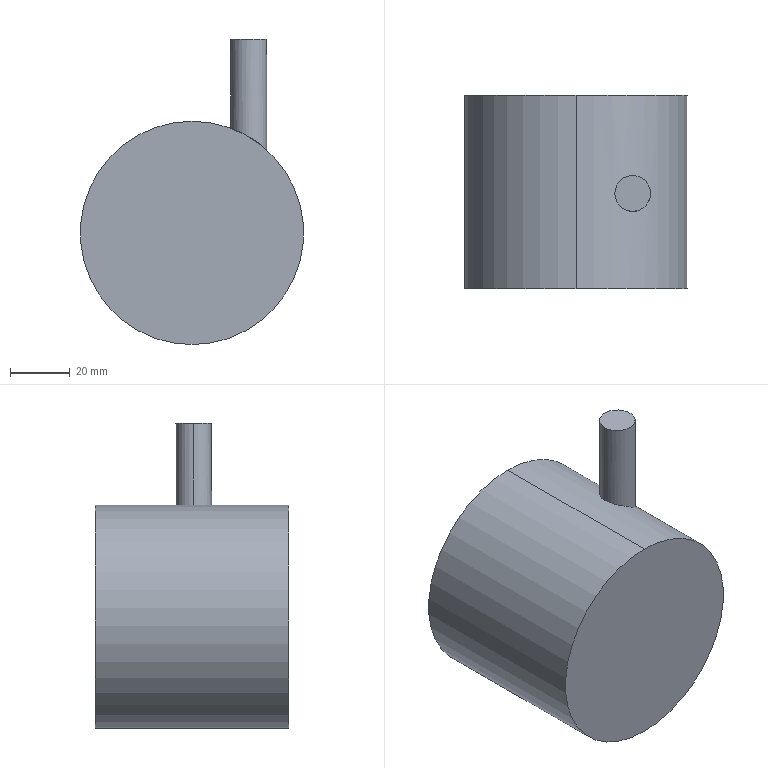Part | SolidWorks | features Extrusion 1, ICE 1 | 1 solid | 7 faces | box 75 x 65 x 102.5 mm | volume 290882 mm3 | cylinder 4 | plane 3 | commonest cylinder face diameters 12 x2 75 x2
STEP:
#1=CARTESIAN_POINT('',(25.06,31.933,65.));
#2=VERTEX_POINT('',#1);
#3=CARTESIAN_POINT('',(13.06,31.933,65.));
#4=VERTEX_POINT('',#3);
#5=CARTESIAN_POINT('',(19.06,31.933,65.));
#6=DIRECTION('',(0.,0.,1.));
#7=DIRECTION('',(1.,0.,0.));
#8=AXIS2_PLACEMENT_3D('',#5,#6,#7);
#9=CIRCLE('',#8,6.);
#10=EDGE_CURVE('',#2,#4,#9,.T.);
#11=ORIENTED_EDGE('',*,*,#10,.F.);
#12=CARTESIAN_POINT('',(25.06,31.933,27.897));
#13=VERTEX_POINT('',#12);
#14=CARTESIAN_POINT('',(25.06,31.933,65.));
#15=DIRECTION('',(0.,0.,-1.));
#16=VECTOR('',#15,1000.);
#17=LINE('',#14,#16);
#18=EDGE_CURVE('',#2,#13,#17,.T.);
#19=ORIENTED_EDGE('',*,*,#18,.T.);
#20=CARTESIAN_POINT('',(13.06,31.933,35.152));
#21=VERTEX_POINT('',#20);
#22=CARTESIAN_POINT('',(25.06,31.933,27.897));
#23=CARTESIAN_POINT('',(25.06,32.147,27.897));
#24=CARTESIAN_POINT('',(25.048,32.362,27.907));
#25=CARTESIAN_POINT('',(25.003,32.789,27.949));
#26=CARTESIAN_POINT('',(24.969,32.998,27.979));
#27=CARTESIAN_POINT('',(24.835,33.613,28.097));
#28=CARTESIAN_POINT('',(24.703,34.011,28.214));
#29=CARTESIAN_POINT('',(24.456,34.564,28.428));
#30=CARTESIAN_POINT('',(24.366,34.742,28.506));
#31=CARTESIAN_POINT('',(24.17,35.085,28.672));
#32=CARTESIAN_POINT('',(24.063,35.251,28.762));
#33=CARTESIAN_POINT('',(23.727,35.724,29.041));
#34=CARTESIAN_POINT('',(23.481,36.007,29.241));
#35=CARTESIAN_POINT('',(22.947,36.519,29.662));
#36=CARTESIAN_POINT('',(22.656,36.75,29.884));
#37=CARTESIAN_POINT('',(22.048,37.149,30.336));
#38=CARTESIAN_POINT('',(21.731,37.318,30.564));
#39=CARTESIAN_POINT('',(21.069,37.599,31.024));
#40=CARTESIAN_POINT('',(20.722,37.71,31.258));
#41=CARTESIAN_POINT('',(20.017,37.868,31.713));
#42=CARTESIAN_POINT('',(19.659,37.915,31.937));
#43=CARTESIAN_POINT('',(19.113,37.936,32.264));
#44=CARTESIAN_POINT('',(18.93,37.935,32.372));
#45=CARTESIAN_POINT('',(18.56,37.915,32.586));
#46=CARTESIAN_POINT('',(18.372,37.897,32.692));
#47=CARTESIAN_POINT('',(17.815,37.815,33.001));
#48=CARTESIAN_POINT('',(17.448,37.726,33.196));
#49=CARTESIAN_POINT('',(16.728,37.475,33.564));
#50=CARTESIAN_POINT('',(16.373,37.313,33.739));
#51=CARTESIAN_POINT('',(15.685,36.91,34.065));
#52=CARTESIAN_POINT('',(15.361,36.675,34.211));
#53=CARTESIAN_POINT('',(14.91,36.272,34.409));
#54=CARTESIAN_POINT('',(14.766,36.129,34.471));
#55=CARTESIAN_POINT('',(14.489,35.825,34.588));
#56=CARTESIAN_POINT('',(14.356,35.663,34.644));
#57=CARTESIAN_POINT('',(13.984,35.159,34.796));
#58=CARTESIAN_POINT('',(13.772,34.8,34.88));
#59=CARTESIAN_POINT('',(13.424,34.033,35.016));
#60=CARTESIAN_POINT('',(13.287,33.621,35.067));
#61=CARTESIAN_POINT('',(13.106,32.79,35.135));
#62=CARTESIAN_POINT('',(13.06,32.365,35.152));
#63=CARTESIAN_POINT('',(13.06,31.933,35.152));
#64=B_SPLINE_CURVE_WITH_KNOTS('',3,(#22,#23,#24,#25,#26,#27,#28,#29,#30,#31,#32,#33,#34,#35,#36,#37,#38,#39,#40,#41,#42,#43,#44,#45,#46,#47,#48,#49,#50,#51,#52,#53,#54,#55,#56,#57,#58,#59,#60,#61,#62,#63),.UNSPECIFIED.,.F.,.F.,(4,2,2,2,2,2,2,2,2,2,2,2,2,2,2,2,2,2,2,2,4),(0.02042,0.02106,0.0217,0.02298,0.02361,0.02425,0.02553,0.0268,0.02808,0.02936,0.03063,0.03127,0.03191,0.03319,0.03446,0.03574,0.03638,0.03701,0.03829,0.03957,0.04084),.UNSPECIFIED.);
#65=EDGE_CURVE('',#13,#21,#64,.T.);
#66=ORIENTED_EDGE('',*,*,#65,.T.);
#67=CARTESIAN_POINT('',(13.06,31.933,65.));
#68=DIRECTION('',(0.,0.,-1.));
#69=VECTOR('',#68,1000.);
#70=LINE('',#67,#69);
#71=EDGE_CURVE('',#4,#21,#70,.T.);
#72=ORIENTED_EDGE('',*,*,#71,.F.);
#73=EDGE_LOOP('',(#11,#19,#66,#72));
#74=FACE_OUTER_BOUND('',#73,.T.);
#75=CARTESIAN_POINT('',(19.06,31.933,65.));
#76=DIRECTION('',(0.,0.,-1.));
#77=DIRECTION('',(-1.,0.,0.));
#78=AXIS2_PLACEMENT_3D('',#75,#76,#77);
#79=CYLINDRICAL_SURFACE('',#78,6.);
#80=ADVANCED_FACE('',(#74),#79,.T.);
#81=CARTESIAN_POINT('',(13.06,31.933,35.152));
#82=CARTESIAN_POINT('',(13.06,31.502,35.152));
#83=CARTESIAN_POINT('',(13.106,31.078,35.135));
#84=CARTESIAN_POINT('',(13.286,30.248,35.068));
#85=CARTESIAN_POINT('',(13.422,29.837,35.016));
#86=CARTESIAN_POINT('',(13.77,29.071,34.881));
#87=CARTESIAN_POINT('',(13.982,28.71,34.797));
#88=CARTESIAN_POINT('',(14.48,28.035,34.593));
#89=CARTESIAN_POINT('',(14.757,27.733,34.476));
#90=CARTESIAN_POINT('',(15.361,27.192,34.211));
#91=CARTESIAN_POINT('',(15.691,26.953,34.061));
#92=CARTESIAN_POINT('',(16.373,26.554,33.739));
#93=CARTESIAN_POINT('',(16.727,26.392,33.565));
#94=CARTESIAN_POINT('',(17.458,26.138,33.191));
#95=CARTESIAN_POINT('',(17.829,26.049,32.993));
#96=CARTESIAN_POINT('',(18.568,25.942,32.583));
#97=CARTESIAN_POINT('',(18.94,25.923,32.369));
#98=CARTESIAN_POINT('',(19.675,25.954,31.927));
#99=CARTESIAN_POINT('',(20.034,26.002,31.703));
#100=CARTESIAN_POINT('',(20.736,26.161,31.248));
#101=CARTESIAN_POINT('',(21.081,26.272,31.016));
#102=CARTESIAN_POINT('',(21.745,26.556,30.554));
#103=CARTESIAN_POINT('',(22.061,26.725,30.326));
#104=CARTESIAN_POINT('',(22.663,27.122,29.879));
#105=CARTESIAN_POINT('',(22.949,27.349,29.66));
#106=CARTESIAN_POINT('',(23.489,27.868,29.234));
#107=CARTESIAN_POINT('',(23.735,28.154,29.034));
#108=CARTESIAN_POINT('',(24.068,28.624,28.758));
#109=CARTESIAN_POINT('',(24.173,28.787,28.67));
#110=CARTESIAN_POINT('',(24.369,29.131,28.503));
#111=CARTESIAN_POINT('',(24.46,29.311,28.425));
#112=CARTESIAN_POINT('',(24.706,29.864,28.211));
#113=CARTESIAN_POINT('',(24.836,30.254,28.097));
#114=CARTESIAN_POINT('',(25.015,31.084,27.938));
#115=CARTESIAN_POINT('',(25.06,31.507,27.897));
#116=CARTESIAN_POINT('',(25.06,31.933,27.897));
#117=B_SPLINE_CURVE_WITH_KNOTS('',3,(#81,#82,#83,#84,#85,#86,#87,#88,#89,#90,#91,#92,#93,#94,#95,#96,#97,#98,#99,#100,#101,#102,#103,#104,#105,#106,#107,#108,#109,#110,#111,#112,#113,#114,#115,#116),.UNSPECIFIED.,.F.,.F.,(4,2,2,2,2,2,2,2,2,2,2,2,2,2,2,2,2,4),(0.,0.001277,0.002553,0.00383,0.005106,0.006383,0.007659,0.008936,0.01021,0.01149,0.01277,0.01404,0.01532,0.01659,0.01723,0.01787,0.01915,0.02042),.UNSPECIFIED.);
#118=EDGE_CURVE('',#21,#13,#117,.T.);
#119=ORIENTED_EDGE('',*,*,#118,.F.);
#120=ORIENTED_EDGE('',*,*,#65,.F.);
#121=EDGE_LOOP('',(#119,#120));
#122=FACE_BOUND('',#121,.T.);
#123=CARTESIAN_POINT('',(0.,65.,37.5));
#124=VERTEX_POINT('',#123);
#125=CARTESIAN_POINT('',(0.,65.,-37.5));
#126=VERTEX_POINT('',#125);
#127=CARTESIAN_POINT('',(0.,65.,0.));
#128=DIRECTION('',(0.,1.,0.));
#129=DIRECTION('',(0.,0.,1.));
#130=AXIS2_PLACEMENT_3D('',#127,#128,#129);
#131=CIRCLE('',#130,37.5);
#132=EDGE_CURVE('',#124,#126,#131,.T.);
#133=ORIENTED_EDGE('',*,*,#132,.F.);
#134=CARTESIAN_POINT('',(0.,0.,37.5));
#135=VERTEX_POINT('',#134);
#136=CARTESIAN_POINT('',(0.,65.,37.5));
#137=DIRECTION('',(0.,-1.,0.));
#138=VECTOR('',#137,1000.);
#139=LINE('',#136,#138);
#140=EDGE_CURVE('',#124,#135,#139,.T.);
#141=ORIENTED_EDGE('',*,*,#140,.T.);
#142=CARTESIAN_POINT('',(0.,0.,-37.5));
#143=VERTEX_POINT('',#142);
#144=CARTESIAN_POINT('',(0.,0.,0.));
#145=DIRECTION('',(0.,1.,0.));
#146=DIRECTION('',(0.,0.,1.));
#147=AXIS2_PLACEMENT_3D('',#144,#145,#146);
#148=CIRCLE('',#147,37.5);
#149=EDGE_CURVE('',#135,#143,#148,.T.);
#150=ORIENTED_EDGE('',*,*,#149,.T.);
#151=CARTESIAN_POINT('',(0.,65.,-37.5));
#152=DIRECTION('',(0.,-1.,0.));
#153=VECTOR('',#152,1000.);
#154=LINE('',#151,#153);
#155=EDGE_CURVE('',#126,#143,#154,.T.);
#156=ORIENTED_EDGE('',*,*,#155,.F.);
#157=EDGE_LOOP('',(#133,#141,#150,#156));
#158=FACE_OUTER_BOUND('',#157,.T.);
#159=CARTESIAN_POINT('',(0.,65.,0.));
#160=DIRECTION('',(0.,-1.,0.));
#161=DIRECTION('',(0.,0.,-1.));
#162=AXIS2_PLACEMENT_3D('',#159,#160,#161);
#163=CYLINDRICAL_SURFACE('',#162,37.5);
#164=ADVANCED_FACE('',(#122,#158),#163,.T.);
#165=ORIENTED_EDGE('',*,*,#140,.F.);
#166=CARTESIAN_POINT('',(0.,65.,0.));
#167=DIRECTION('',(0.,1.,0.));
#168=DIRECTION('',(0.,0.,1.));
#169=AXIS2_PLACEMENT_3D('',#166,#167,#168);
#170=CIRCLE('',#169,37.5);
#171=EDGE_CURVE('',#126,#124,#170,.T.);
#172=ORIENTED_EDGE('',*,*,#171,.F.);
#173=ORIENTED_EDGE('',*,*,#155,.T.);
#174=CARTESIAN_POINT('',(0.,0.,0.));
#175=DIRECTION('',(0.,1.,0.));
#176=DIRECTION('',(0.,0.,1.));
#177=AXIS2_PLACEMENT_3D('',#174,#175,#176);
#178=CIRCLE('',#177,37.5);
#179=EDGE_CURVE('',#143,#135,#178,.T.);
#180=ORIENTED_EDGE('',*,*,#179,.T.);
#181=EDGE_LOOP('',(#165,#172,#173,#180));
#182=FACE_OUTER_BOUND('',#181,.T.);
#183=CARTESIAN_POINT('',(0.,65.,0.));
#184=DIRECTION('',(0.,-1.,0.));
#185=DIRECTION('',(0.,0.,-1.));
#186=AXIS2_PLACEMENT_3D('',#183,#184,#185);
#187=CYLINDRICAL_SURFACE('',#186,37.5);
#188=ADVANCED_FACE('',(#182),#187,.T.);
#189=ORIENTED_EDGE('',*,*,#171,.T.);
#190=ORIENTED_EDGE('',*,*,#132,.T.);
#191=EDGE_LOOP('',(#189,#190));
#192=FACE_OUTER_BOUND('',#191,.T.);
#193=CARTESIAN_POINT('',(0.,65.,0.));
#194=DIRECTION('',(0.,1.,0.));
#195=DIRECTION('',(0.,0.,1.));
#196=AXIS2_PLACEMENT_3D('',#193,#194,#195);
#197=PLANE('',#196);
#198=ADVANCED_FACE('',(#192),#197,.T.);
#199=ORIENTED_EDGE('',*,*,#179,.F.);
#200=ORIENTED_EDGE('',*,*,#149,.F.);
#201=EDGE_LOOP('',(#199,#200));
#202=FACE_OUTER_BOUND('',#201,.T.);
#203=CARTESIAN_POINT('',(0.,0.,0.));
#204=DIRECTION('',(0.,1.,0.));
#205=DIRECTION('',(0.,0.,1.));
#206=AXIS2_PLACEMENT_3D('',#203,#204,#205);
#207=PLANE('',#206);
#208=ADVANCED_FACE('',(#202),#207,.F.);
#209=ORIENTED_EDGE('',*,*,#18,.F.);
#210=CARTESIAN_POINT('',(19.06,31.933,65.));
#211=DIRECTION('',(0.,0.,1.));
#212=DIRECTION('',(1.,0.,0.));
#213=AXIS2_PLACEMENT_3D('',#210,#211,#212);
#214=CIRCLE('',#213,6.);
#215=EDGE_CURVE('',#4,#2,#214,.T.);
#216=ORIENTED_EDGE('',*,*,#215,.F.);
#217=ORIENTED_EDGE('',*,*,#71,.T.);
#218=ORIENTED_EDGE('',*,*,#118,.T.);
#219=EDGE_LOOP('',(#209,#216,#217,#218));
#220=FACE_OUTER_BOUND('',#219,.T.);
#221=CARTESIAN_POINT('',(19.06,31.933,65.));
#222=DIRECTION('',(0.,0.,-1.));
#223=DIRECTION('',(-1.,0.,0.));
#224=AXIS2_PLACEMENT_3D('',#221,#222,#223);
#225=CYLINDRICAL_SURFACE('',#224,6.);
#226=ADVANCED_FACE('',(#220),#225,.T.);
#227=ORIENTED_EDGE('',*,*,#215,.T.);
#228=ORIENTED_EDGE('',*,*,#10,.T.);
#229=EDGE_LOOP('',(#227,#228));
#230=FACE_OUTER_BOUND('',#229,.T.);
#231=CARTESIAN_POINT('',(19.06,31.933,65.));
#232=DIRECTION('',(0.,0.,1.));
#233=DIRECTION('',(1.,0.,0.));
#234=AXIS2_PLACEMENT_3D('',#231,#232,#233);
#235=PLANE('',#234);
#236=ADVANCED_FACE('',(#230),#235,.T.);
#237=CLOSED_SHELL('',(#80,#164,#188,#198,#208,#226,#236));
#238=MANIFOLD_SOLID_BREP('',#237);
#239=CARTESIAN_POINT('',(0.,0.,0.));
#240=DIRECTION('',(0.,0.,1.));
#241=DIRECTION('',(1.,0.,0.));
#242=AXIS2_PLACEMENT_3D('',#239,#240,#241);
#243=(LENGTH_UNIT()NAMED_UNIT(*)SI_UNIT(.MILLI.,.METRE.));
#244=UNCERTAINTY_MEASURE_WITH_UNIT(LENGTH_MEASURE(0.00001),#243,'','');
#245=(NAMED_UNIT(*)PLANE_ANGLE_UNIT()SI_UNIT($,.RADIAN.));
#246=(NAMED_UNIT(*)SI_UNIT($,.STERADIAN.)SOLID_ANGLE_UNIT());
#247=(GEOMETRIC_REPRESENTATION_CONTEXT(3)GLOBAL_UNCERTAINTY_ASSIGNED_CONTEXT((#244))GLOBAL_UNIT_ASSIGNED_CONTEXT((#243,#245,#246))REPRESENTATION_CONTEXT('',''));
#248=ADVANCED_BREP_SHAPE_REPRESENTATION('',(#238,#242),#247);